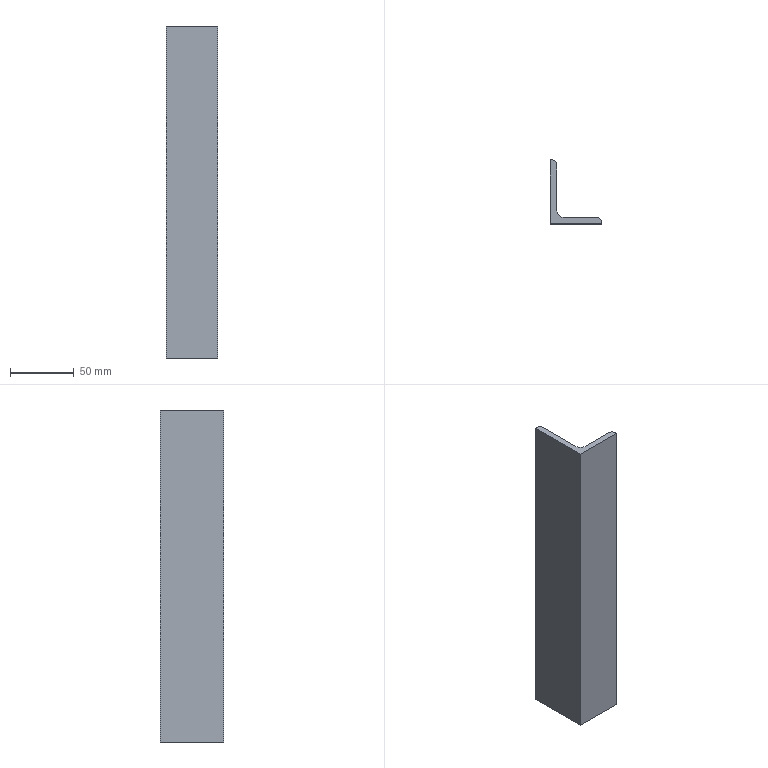Part | STEP file | ISO 657-2 50x 40x 5 1784900831893 | 1 solid | 11 faces | box 40 x 50 x 260 mm | volume 110109 mm3 | plane 8 | cylinder 3 | commonest cylinder face diameters 8 x2 10 x1
STEP:
#1=CARTESIAN_POINT('',(25.4,-10.5,305.));
#2=VERTEX_POINT('',#1);
#3=CARTESIAN_POINT('',(29.4,-14.5,305.));
#4=VERTEX_POINT('',#3);
#5=CARTESIAN_POINT('',(25.4,-14.5,305.));
#6=DIRECTION('',(0.,0.,-1.));
#7=DIRECTION('',(1.,0.,0.));
#8=AXIS2_PLACEMENT_3D('',#5,#6,#7);
#9=CIRCLE('',#8,4.);
#10=EDGE_CURVE('',#2,#4,#9,.T.);
#11=ORIENTED_EDGE('',*,*,#10,.T.);
#12=CARTESIAN_POINT('',(29.4,-14.5,45.));
#13=VERTEX_POINT('',#12);
#14=CARTESIAN_POINT('',(29.4,-14.5,0.));
#15=DIRECTION('',(0.,0.,1.));
#16=VECTOR('',#15,10.);
#17=LINE('',#14,#16);
#18=EDGE_CURVE('',#13,#4,#17,.T.);
#19=ORIENTED_EDGE('',*,*,#18,.F.);
#20=CARTESIAN_POINT('',(25.4,-10.5,45.));
#21=VERTEX_POINT('',#20);
#22=CARTESIAN_POINT('',(25.4,-14.5,45.));
#23=DIRECTION('',(0.,0.,-1.));
#24=DIRECTION('',(1.,0.,0.));
#25=AXIS2_PLACEMENT_3D('',#22,#23,#24);
#26=CIRCLE('',#25,4.);
#27=EDGE_CURVE('',#21,#13,#26,.T.);
#28=ORIENTED_EDGE('',*,*,#27,.F.);
#29=CARTESIAN_POINT('',(25.4,-10.5,0.));
#30=DIRECTION('',(0.,0.,1.));
#31=VECTOR('',#30,10.);
#32=LINE('',#29,#31);
#33=EDGE_CURVE('',#21,#2,#32,.T.);
#34=ORIENTED_EDGE('',*,*,#33,.T.);
#35=EDGE_LOOP('',(#11,#19,#28,#34));
#36=FACE_OUTER_BOUND('',#35,.T.);
#37=CARTESIAN_POINT('',(25.4,-14.5,0.));
#38=DIRECTION('',(0.,0.,1.));
#39=DIRECTION('',(1.,0.,0.));
#40=AXIS2_PLACEMENT_3D('',#37,#38,#39);
#41=CYLINDRICAL_SURFACE('',#40,4.);
#42=ADVANCED_FACE('',(#36),#41,.T.);
#43=CARTESIAN_POINT('',(29.4,-15.5,305.));
#44=VERTEX_POINT('',#43);
#45=CARTESIAN_POINT('',(29.4,-2.5,305.));
#46=DIRECTION('',(0.,-1.,0.));
#47=VECTOR('',#46,10.);
#48=LINE('',#45,#47);
#49=EDGE_CURVE('',#4,#44,#48,.T.);
#50=ORIENTED_EDGE('',*,*,#49,.T.);
#51=CARTESIAN_POINT('',(29.4,-15.5,45.));
#52=VERTEX_POINT('',#51);
#53=CARTESIAN_POINT('',(29.4,-15.5,0.));
#54=DIRECTION('',(0.,0.,1.));
#55=VECTOR('',#54,10.);
#56=LINE('',#53,#55);
#57=EDGE_CURVE('',#52,#44,#56,.T.);
#58=ORIENTED_EDGE('',*,*,#57,.F.);
#59=CARTESIAN_POINT('',(29.4,-2.5,45.));
#60=DIRECTION('',(0.,-1.,0.));
#61=VECTOR('',#60,10.);
#62=LINE('',#59,#61);
#63=EDGE_CURVE('',#13,#52,#62,.T.);
#64=ORIENTED_EDGE('',*,*,#63,.F.);
#65=ORIENTED_EDGE('',*,*,#18,.T.);
#66=EDGE_LOOP('',(#50,#58,#64,#65));
#67=FACE_OUTER_BOUND('',#66,.T.);
#68=CARTESIAN_POINT('',(29.4,-14.5,0.));
#69=DIRECTION('',(1.,0.,0.));
#70=DIRECTION('',(0.,0.,-1.));
#71=AXIS2_PLACEMENT_3D('',#68,#69,#70);
#72=PLANE('',#71);
#73=ADVANCED_FACE('',(#67),#72,.T.);
#74=CARTESIAN_POINT('',(-10.6,-15.5,305.));
#75=VERTEX_POINT('',#74);
#76=CARTESIAN_POINT('',(19.4,-15.5,305.));
#77=DIRECTION('',(-1.,0.,0.));
#78=VECTOR('',#77,10.);
#79=LINE('',#76,#78);
#80=EDGE_CURVE('',#44,#75,#79,.T.);
#81=ORIENTED_EDGE('',*,*,#80,.T.);
#82=CARTESIAN_POINT('',(-10.6,-15.5,45.));
#83=VERTEX_POINT('',#82);
#84=CARTESIAN_POINT('',(-10.6,-15.5,0.));
#85=DIRECTION('',(0.,0.,1.));
#86=VECTOR('',#85,10.);
#87=LINE('',#84,#86);
#88=EDGE_CURVE('',#83,#75,#87,.T.);
#89=ORIENTED_EDGE('',*,*,#88,.F.);
#90=CARTESIAN_POINT('',(19.4,-15.5,45.));
#91=DIRECTION('',(-1.,0.,0.));
#92=VECTOR('',#91,10.);
#93=LINE('',#90,#92);
#94=EDGE_CURVE('',#52,#83,#93,.T.);
#95=ORIENTED_EDGE('',*,*,#94,.F.);
#96=ORIENTED_EDGE('',*,*,#57,.T.);
#97=EDGE_LOOP('',(#81,#89,#95,#96));
#98=FACE_OUTER_BOUND('',#97,.T.);
#99=CARTESIAN_POINT('',(29.4,-15.5,0.));
#100=DIRECTION('',(0.,-1.,0.));
#101=DIRECTION('',(0.,0.,-1.));
#102=AXIS2_PLACEMENT_3D('',#99,#100,#101);
#103=PLANE('',#102);
#104=ADVANCED_FACE('',(#98),#103,.T.);
#105=CARTESIAN_POINT('',(-10.6,34.5,305.));
#106=VERTEX_POINT('',#105);
#107=CARTESIAN_POINT('',(-10.6,-3.,305.));
#108=DIRECTION('',(0.,1.,0.));
#109=VECTOR('',#108,10.);
#110=LINE('',#107,#109);
#111=EDGE_CURVE('',#75,#106,#110,.T.);
#112=ORIENTED_EDGE('',*,*,#111,.T.);
#113=CARTESIAN_POINT('',(-10.6,34.5,45.));
#114=VERTEX_POINT('',#113);
#115=CARTESIAN_POINT('',(-10.6,34.5,0.));
#116=DIRECTION('',(0.,0.,1.));
#117=VECTOR('',#116,10.);
#118=LINE('',#115,#117);
#119=EDGE_CURVE('',#114,#106,#118,.T.);
#120=ORIENTED_EDGE('',*,*,#119,.F.);
#121=CARTESIAN_POINT('',(-10.6,-3.,45.));
#122=DIRECTION('',(0.,1.,0.));
#123=VECTOR('',#122,10.);
#124=LINE('',#121,#123);
#125=EDGE_CURVE('',#83,#114,#124,.T.);
#126=ORIENTED_EDGE('',*,*,#125,.F.);
#127=ORIENTED_EDGE('',*,*,#88,.T.);
#128=EDGE_LOOP('',(#112,#120,#126,#127));
#129=FACE_OUTER_BOUND('',#128,.T.);
#130=CARTESIAN_POINT('',(-10.6,-15.5,0.));
#131=DIRECTION('',(-1.,0.,0.));
#132=DIRECTION('',(0.,0.,1.));
#133=AXIS2_PLACEMENT_3D('',#130,#131,#132);
#134=PLANE('',#133);
#135=ADVANCED_FACE('',(#129),#134,.T.);
#136=CARTESIAN_POINT('',(-9.6,34.5,305.));
#137=VERTEX_POINT('',#136);
#138=CARTESIAN_POINT('',(-0.6,34.5,305.));
#139=DIRECTION('',(1.,0.,0.));
#140=VECTOR('',#139,10.);
#141=LINE('',#138,#140);
#142=EDGE_CURVE('',#106,#137,#141,.T.);
#143=ORIENTED_EDGE('',*,*,#142,.T.);
#144=CARTESIAN_POINT('',(-9.6,34.5,45.));
#145=VERTEX_POINT('',#144);
#146=CARTESIAN_POINT('',(-9.6,34.5,0.));
#147=DIRECTION('',(0.,0.,1.));
#148=VECTOR('',#147,10.);
#149=LINE('',#146,#148);
#150=EDGE_CURVE('',#145,#137,#149,.T.);
#151=ORIENTED_EDGE('',*,*,#150,.F.);
#152=CARTESIAN_POINT('',(-0.6,34.5,45.));
#153=DIRECTION('',(1.,0.,0.));
#154=VECTOR('',#153,10.);
#155=LINE('',#152,#154);
#156=EDGE_CURVE('',#114,#145,#155,.T.);
#157=ORIENTED_EDGE('',*,*,#156,.F.);
#158=ORIENTED_EDGE('',*,*,#119,.T.);
#159=EDGE_LOOP('',(#143,#151,#157,#158));
#160=FACE_OUTER_BOUND('',#159,.T.);
#161=CARTESIAN_POINT('',(-10.6,34.5,0.));
#162=DIRECTION('',(0.,1.,0.));
#163=DIRECTION('',(0.,0.,1.));
#164=AXIS2_PLACEMENT_3D('',#161,#162,#163);
#165=PLANE('',#164);
#166=ADVANCED_FACE('',(#160),#165,.T.);
#167=CARTESIAN_POINT('',(-5.6,30.5,305.));
#168=VERTEX_POINT('',#167);
#169=CARTESIAN_POINT('',(-9.6,30.5,305.));
#170=DIRECTION('',(0.,0.,-1.));
#171=DIRECTION('',(1.,0.,0.));
#172=AXIS2_PLACEMENT_3D('',#169,#170,#171);
#173=CIRCLE('',#172,4.);
#174=EDGE_CURVE('',#137,#168,#173,.T.);
#175=ORIENTED_EDGE('',*,*,#174,.T.);
#176=CARTESIAN_POINT('',(-5.6,30.5,45.));
#177=VERTEX_POINT('',#176);
#178=CARTESIAN_POINT('',(-5.6,30.5,0.));
#179=DIRECTION('',(0.,0.,1.));
#180=VECTOR('',#179,10.);
#181=LINE('',#178,#180);
#182=EDGE_CURVE('',#177,#168,#181,.T.);
#183=ORIENTED_EDGE('',*,*,#182,.F.);
#184=CARTESIAN_POINT('',(-9.6,30.5,45.));
#185=DIRECTION('',(0.,0.,-1.));
#186=DIRECTION('',(1.,0.,0.));
#187=AXIS2_PLACEMENT_3D('',#184,#185,#186);
#188=CIRCLE('',#187,4.);
#189=EDGE_CURVE('',#145,#177,#188,.T.);
#190=ORIENTED_EDGE('',*,*,#189,.F.);
#191=ORIENTED_EDGE('',*,*,#150,.T.);
#192=EDGE_LOOP('',(#175,#183,#190,#191));
#193=FACE_OUTER_BOUND('',#192,.T.);
#194=CARTESIAN_POINT('',(-9.6,30.5,0.));
#195=DIRECTION('',(0.,0.,1.));
#196=DIRECTION('',(1.,0.,0.));
#197=AXIS2_PLACEMENT_3D('',#194,#195,#196);
#198=CYLINDRICAL_SURFACE('',#197,4.);
#199=ADVANCED_FACE('',(#193),#198,.T.);
#200=CARTESIAN_POINT('',(-5.6,-5.5,305.));
#201=VERTEX_POINT('',#200);
#202=CARTESIAN_POINT('',(-5.6,20.,305.));
#203=DIRECTION('',(0.,-1.,0.));
#204=VECTOR('',#203,10.);
#205=LINE('',#202,#204);
#206=EDGE_CURVE('',#168,#201,#205,.T.);
#207=ORIENTED_EDGE('',*,*,#206,.T.);
#208=CARTESIAN_POINT('',(-5.6,-5.5,45.));
#209=VERTEX_POINT('',#208);
#210=CARTESIAN_POINT('',(-5.6,-5.5,0.));
#211=DIRECTION('',(0.,0.,1.));
#212=VECTOR('',#211,10.);
#213=LINE('',#210,#212);
#214=EDGE_CURVE('',#209,#201,#213,.T.);
#215=ORIENTED_EDGE('',*,*,#214,.F.);
#216=CARTESIAN_POINT('',(-5.6,20.,45.));
#217=DIRECTION('',(0.,-1.,0.));
#218=VECTOR('',#217,10.);
#219=LINE('',#216,#218);
#220=EDGE_CURVE('',#177,#209,#219,.T.);
#221=ORIENTED_EDGE('',*,*,#220,.F.);
#222=ORIENTED_EDGE('',*,*,#182,.T.);
#223=EDGE_LOOP('',(#207,#215,#221,#222));
#224=FACE_OUTER_BOUND('',#223,.T.);
#225=CARTESIAN_POINT('',(-5.6,30.5,0.));
#226=DIRECTION('',(1.,0.,0.));
#227=DIRECTION('',(0.,0.,-1.));
#228=AXIS2_PLACEMENT_3D('',#225,#226,#227);
#229=PLANE('',#228);
#230=ADVANCED_FACE('',(#224),#229,.T.);
#231=CARTESIAN_POINT('',(-0.6,-10.5,305.));
#232=VERTEX_POINT('',#231);
#233=CARTESIAN_POINT('',(-0.6,-5.5,305.));
#234=DIRECTION('',(0.,0.,1.));
#235=DIRECTION('',(1.,0.,0.));
#236=AXIS2_PLACEMENT_3D('',#233,#234,#235);
#237=CIRCLE('',#236,5.);
#238=EDGE_CURVE('',#201,#232,#237,.T.);
#239=ORIENTED_EDGE('',*,*,#238,.T.);
#240=CARTESIAN_POINT('',(-0.6,-10.5,45.));
#241=VERTEX_POINT('',#240);
#242=CARTESIAN_POINT('',(-0.6,-10.5,0.));
#243=DIRECTION('',(0.,0.,1.));
#244=VECTOR('',#243,10.);
#245=LINE('',#242,#244);
#246=EDGE_CURVE('',#241,#232,#245,.T.);
#247=ORIENTED_EDGE('',*,*,#246,.F.);
#248=CARTESIAN_POINT('',(-0.6,-5.5,45.));
#249=DIRECTION('',(0.,0.,1.));
#250=DIRECTION('',(1.,0.,0.));
#251=AXIS2_PLACEMENT_3D('',#248,#249,#250);
#252=CIRCLE('',#251,5.);
#253=EDGE_CURVE('',#209,#241,#252,.T.);
#254=ORIENTED_EDGE('',*,*,#253,.F.);
#255=ORIENTED_EDGE('',*,*,#214,.T.);
#256=EDGE_LOOP('',(#239,#247,#254,#255));
#257=FACE_OUTER_BOUND('',#256,.T.);
#258=CARTESIAN_POINT('',(-0.6,-5.5,0.));
#259=DIRECTION('',(0.,0.,1.));
#260=DIRECTION('',(1.,0.,0.));
#261=AXIS2_PLACEMENT_3D('',#258,#259,#260);
#262=CYLINDRICAL_SURFACE('',#261,5.);
#263=ADVANCED_FACE('',(#257),#262,.F.);
#264=CARTESIAN_POINT('',(4.4,-10.5,305.));
#265=DIRECTION('',(1.,0.,0.));
#266=VECTOR('',#265,10.);
#267=LINE('',#264,#266);
#268=EDGE_CURVE('',#232,#2,#267,.T.);
#269=ORIENTED_EDGE('',*,*,#268,.T.);
#270=ORIENTED_EDGE('',*,*,#33,.F.);
#271=CARTESIAN_POINT('',(4.4,-10.5,45.));
#272=DIRECTION('',(1.,0.,0.));
#273=VECTOR('',#272,10.);
#274=LINE('',#271,#273);
#275=EDGE_CURVE('',#241,#21,#274,.T.);
#276=ORIENTED_EDGE('',*,*,#275,.F.);
#277=ORIENTED_EDGE('',*,*,#246,.T.);
#278=EDGE_LOOP('',(#269,#270,#276,#277));
#279=FACE_OUTER_BOUND('',#278,.T.);
#280=CARTESIAN_POINT('',(-0.6,-10.5,0.));
#281=DIRECTION('',(0.,1.,0.));
#282=DIRECTION('',(0.,0.,1.));
#283=AXIS2_PLACEMENT_3D('',#280,#281,#282);
#284=PLANE('',#283);
#285=ADVANCED_FACE('',(#279),#284,.T.);
#286=ORIENTED_EDGE('',*,*,#156,.T.);
#287=ORIENTED_EDGE('',*,*,#189,.T.);
#288=ORIENTED_EDGE('',*,*,#220,.T.);
#289=ORIENTED_EDGE('',*,*,#253,.T.);
#290=ORIENTED_EDGE('',*,*,#275,.T.);
#291=ORIENTED_EDGE('',*,*,#27,.T.);
#292=ORIENTED_EDGE('',*,*,#63,.T.);
#293=ORIENTED_EDGE('',*,*,#94,.T.);
#294=ORIENTED_EDGE('',*,*,#125,.T.);
#295=EDGE_LOOP('',(#286,#287,#288,#289,#290,#291,#292,#293,#294));
#296=FACE_OUTER_BOUND('',#295,.T.);
#297=CARTESIAN_POINT('',(9.4,9.5,45.));
#298=DIRECTION('',(0.,0.,1.));
#299=DIRECTION('',(1.,0.,0.));
#300=AXIS2_PLACEMENT_3D('',#297,#298,#299);
#301=PLANE('',#300);
#302=ADVANCED_FACE('',(#296),#301,.F.);
#303=ORIENTED_EDGE('',*,*,#142,.F.);
#304=ORIENTED_EDGE('',*,*,#111,.F.);
#305=ORIENTED_EDGE('',*,*,#80,.F.);
#306=ORIENTED_EDGE('',*,*,#49,.F.);
#307=ORIENTED_EDGE('',*,*,#10,.F.);
#308=ORIENTED_EDGE('',*,*,#268,.F.);
#309=ORIENTED_EDGE('',*,*,#238,.F.);
#310=ORIENTED_EDGE('',*,*,#206,.F.);
#311=ORIENTED_EDGE('',*,*,#174,.F.);
#312=EDGE_LOOP('',(#303,#304,#305,#306,#307,#308,#309,#310,#311));
#313=FACE_OUTER_BOUND('',#312,.T.);
#314=CARTESIAN_POINT('',(9.4,9.5,305.));
#315=DIRECTION('',(0.,0.,1.));
#316=DIRECTION('',(1.,0.,0.));
#317=AXIS2_PLACEMENT_3D('',#314,#315,#316);
#318=PLANE('',#317);
#319=ADVANCED_FACE('',(#313),#318,.T.);
#320=CLOSED_SHELL('',(#42,#73,#104,#135,#166,#199,#230,#263,#285,#302,#319));
#321=MANIFOLD_SOLID_BREP('',#320);
#322=(LENGTH_UNIT()NAMED_UNIT(*)SI_UNIT(.MILLI.,.METRE.));
#323=UNCERTAINTY_MEASURE_WITH_UNIT(LENGTH_MEASURE(0.01),#322,'','');
#324=(NAMED_UNIT(*)PLANE_ANGLE_UNIT()SI_UNIT($,.RADIAN.));
#325=(NAMED_UNIT(*)SI_UNIT($,.STERADIAN.)SOLID_ANGLE_UNIT());
#326=(GEOMETRIC_REPRESENTATION_CONTEXT(3)GLOBAL_UNCERTAINTY_ASSIGNED_CONTEXT((#323))GLOBAL_UNIT_ASSIGNED_CONTEXT((#322,#324,#325))REPRESENTATION_CONTEXT('',''));
#327=ADVANCED_BREP_SHAPE_REPRESENTATION('',(#321),#326);